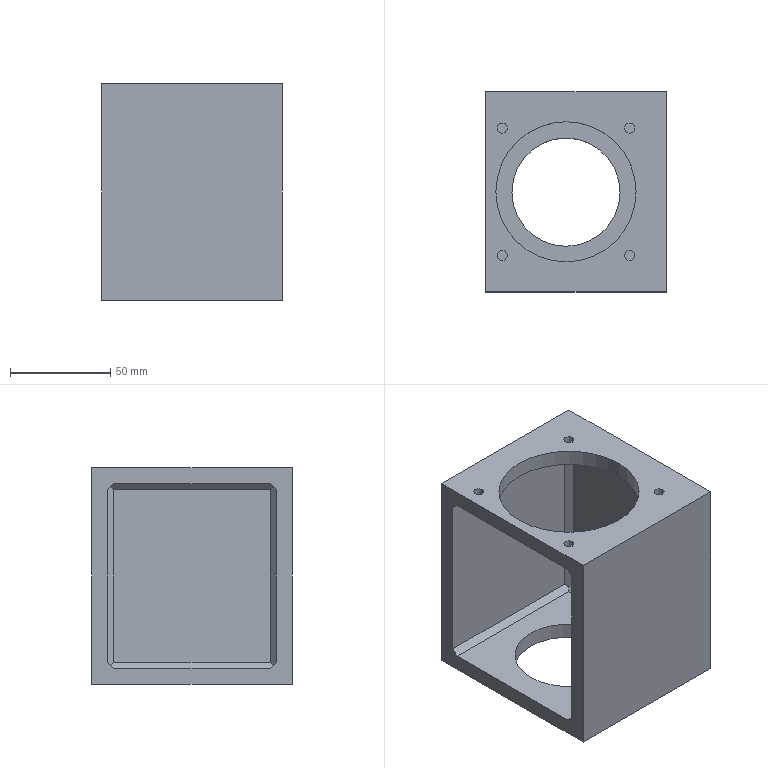Part | Creo | features CURVE 4, DATUM PLANE 3, CUT 2, PROTRUSION 2, CHAMFER 1, COORDINATE SYSTEM 1 | 1 solid | 31 faces | box 90 x 100 x 108 mm | volume 291545 mm3 | plane 19 | cylinder 12 | commonest cylinder face diameters 5 x8 54 x2 70 x2
STEP:
#1=CARTESIAN_POINT('',(0.,0.,0.));
#2=DIRECTION('',(0.,0.,1.));
#3=DIRECTION('',(1.,0.,0.));
#4=AXIS2_PLACEMENT_3D('',#1,#2,#3);
#5=CARTESIAN_POINT('',(-45.,50.,-54.));
#6=VERTEX_POINT('',#5);
#7=CARTESIAN_POINT('',(-45.,-50.,-54.));
#8=VERTEX_POINT('',#7);
#9=CARTESIAN_POINT('',(-45.,50.,-54.));
#10=DIRECTION('',(0.,-1.,0.));
#11=VECTOR('',#10,100.);
#12=LINE('',#9,#11);
#13=EDGE_CURVE('',#6,#8,#12,.T.);
#14=ORIENTED_EDGE('',*,*,#13,.T.);
#15=CARTESIAN_POINT('',(45.,-50.,-54.));
#16=VERTEX_POINT('',#15);
#17=CARTESIAN_POINT('',(-45.,-50.,-54.));
#18=DIRECTION('',(1.,0.,0.));
#19=VECTOR('',#18,90.);
#20=LINE('',#17,#19);
#21=EDGE_CURVE('',#8,#16,#20,.T.);
#22=ORIENTED_EDGE('',*,*,#21,.T.);
#23=CARTESIAN_POINT('',(45.,50.,-54.));
#24=VERTEX_POINT('',#23);
#25=CARTESIAN_POINT('',(45.,-50.,-54.));
#26=DIRECTION('',(0.,1.,0.));
#27=VECTOR('',#26,100.);
#28=LINE('',#25,#27);
#29=EDGE_CURVE('',#16,#24,#28,.T.);
#30=ORIENTED_EDGE('',*,*,#29,.T.);
#31=CARTESIAN_POINT('',(45.,50.,-54.));
#32=DIRECTION('',(-1.,0.,0.));
#33=VECTOR('',#32,90.);
#34=LINE('',#31,#33);
#35=EDGE_CURVE('',#24,#6,#34,.T.);
#36=ORIENTED_EDGE('',*,*,#35,.T.);
#37=EDGE_LOOP('',(#14,#22,#30,#36));
#38=FACE_OUTER_BOUND('',#37,.F.);
#39=CARTESIAN_POINT('',(-32.,0.,-54.));
#40=VERTEX_POINT('',#39);
#41=CARTESIAN_POINT('',(22.,0.,-54.));
#42=VERTEX_POINT('',#41);
#43=CARTESIAN_POINT('',(-5.,0.,-54.));
#44=DIRECTION('',(0.,0.,1.));
#45=DIRECTION('',(-1.,0.,0.));
#46=AXIS2_PLACEMENT_3D('',#43,#44,#45);
#47=CIRCLE('',#46,27.);
#48=EDGE_CURVE('',#40,#42,#47,.T.);
#49=ORIENTED_EDGE('',*,*,#48,.F.);
#50=CARTESIAN_POINT('',(-5.,0.,-54.));
#51=DIRECTION('',(0.,0.,1.));
#52=DIRECTION('',(1.,0.,0.));
#53=AXIS2_PLACEMENT_3D('',#50,#51,#52);
#54=CIRCLE('',#53,27.);
#55=EDGE_CURVE('',#42,#40,#54,.T.);
#56=ORIENTED_EDGE('',*,*,#55,.F.);
#57=EDGE_LOOP('',(#49,#56));
#58=FACE_BOUND('',#57,.F.);
#59=CARTESIAN_POINT('',(0.,0.,-54.));
#60=DIRECTION('',(0.,0.,1.));
#61=DIRECTION('',(1.,0.,0.));
#62=AXIS2_PLACEMENT_3D('',#59,#60,#61);
#63=PLANE('',#62);
#64=ADVANCED_FACE('',(#38,#58),#63,.F.);
#65=ORIENTED_EDGE('',*,*,#48,.T.);
#66=CARTESIAN_POINT('',(22.,0.,-46.));
#67=VERTEX_POINT('',#66);
#68=CARTESIAN_POINT('',(22.,0.,-54.));
#69=DIRECTION('',(0.,0.,1.));
#70=VECTOR('',#69,8.);
#71=LINE('',#68,#70);
#72=EDGE_CURVE('',#42,#67,#71,.T.);
#73=ORIENTED_EDGE('',*,*,#72,.T.);
#74=CARTESIAN_POINT('',(-32.,0.,-46.));
#75=VERTEX_POINT('',#74);
#76=CARTESIAN_POINT('',(-5.,0.,-46.));
#77=DIRECTION('',(0.,0.,1.));
#78=DIRECTION('',(-1.,0.,0.));
#79=AXIS2_PLACEMENT_3D('',#76,#77,#78);
#80=CIRCLE('',#79,27.);
#81=EDGE_CURVE('',#75,#67,#80,.T.);
#82=ORIENTED_EDGE('',*,*,#81,.F.);
#83=CARTESIAN_POINT('',(-32.,0.,-54.));
#84=DIRECTION('',(0.,0.,1.));
#85=VECTOR('',#84,8.);
#86=LINE('',#83,#85);
#87=EDGE_CURVE('',#40,#75,#86,.T.);
#88=ORIENTED_EDGE('',*,*,#87,.F.);
#89=EDGE_LOOP('',(#65,#73,#82,#88));
#90=FACE_OUTER_BOUND('',#89,.F.);
#91=CARTESIAN_POINT('',(-5.,0.,-54.));
#92=DIRECTION('',(0.,0.,-1.));
#93=DIRECTION('',(-1.,0.,0.));
#94=AXIS2_PLACEMENT_3D('',#91,#92,#93);
#95=CYLINDRICAL_SURFACE('',#94,27.);
#96=ADVANCED_FACE('',(#90),#95,.F.);
#97=ORIENTED_EDGE('',*,*,#55,.T.);
#98=ORIENTED_EDGE('',*,*,#87,.T.);
#99=CARTESIAN_POINT('',(-5.,0.,-46.));
#100=DIRECTION('',(0.,0.,1.));
#101=DIRECTION('',(1.,0.,0.));
#102=AXIS2_PLACEMENT_3D('',#99,#100,#101);
#103=CIRCLE('',#102,27.);
#104=EDGE_CURVE('',#67,#75,#103,.T.);
#105=ORIENTED_EDGE('',*,*,#104,.F.);
#106=ORIENTED_EDGE('',*,*,#72,.F.);
#107=EDGE_LOOP('',(#97,#98,#105,#106));
#108=FACE_OUTER_BOUND('',#107,.F.);
#109=CARTESIAN_POINT('',(-5.,0.,-54.));
#110=DIRECTION('',(0.,0.,-1.));
#111=DIRECTION('',(-1.,0.,0.));
#112=AXIS2_PLACEMENT_3D('',#109,#110,#111);
#113=CYLINDRICAL_SURFACE('',#112,27.);
#114=ADVANCED_FACE('',(#108),#113,.F.);
#115=CARTESIAN_POINT('',(-45.,-39.,-46.));
#116=VERTEX_POINT('',#115);
#117=CARTESIAN_POINT('',(34.,-39.,-46.));
#118=VERTEX_POINT('',#117);
#119=CARTESIAN_POINT('',(-45.,-39.,-46.));
#120=DIRECTION('',(1.,0.,0.));
#121=VECTOR('',#120,79.);
#122=LINE('',#119,#121);
#123=EDGE_CURVE('',#116,#118,#122,.T.);
#124=ORIENTED_EDGE('',*,*,#123,.F.);
#125=CARTESIAN_POINT('',(-45.,39.,-46.));
#126=VERTEX_POINT('',#125);
#127=CARTESIAN_POINT('',(-45.,39.,-46.));
#128=DIRECTION('',(0.,-1.,0.));
#129=VECTOR('',#128,78.);
#130=LINE('',#127,#129);
#131=EDGE_CURVE('',#126,#116,#130,.T.);
#132=ORIENTED_EDGE('',*,*,#131,.F.);
#133=CARTESIAN_POINT('',(34.,39.,-46.));
#134=VERTEX_POINT('',#133);
#135=CARTESIAN_POINT('',(-45.,39.,-46.));
#136=DIRECTION('',(1.,0.,0.));
#137=VECTOR('',#136,79.);
#138=LINE('',#135,#137);
#139=EDGE_CURVE('',#126,#134,#138,.T.);
#140=ORIENTED_EDGE('',*,*,#139,.T.);
#141=CARTESIAN_POINT('',(34.,-39.,-46.));
#142=DIRECTION('',(0.,1.,0.));
#143=VECTOR('',#142,78.);
#144=LINE('',#141,#143);
#145=EDGE_CURVE('',#118,#134,#144,.T.);
#146=ORIENTED_EDGE('',*,*,#145,.F.);
#147=EDGE_LOOP('',(#124,#132,#140,#146));
#148=FACE_OUTER_BOUND('',#147,.F.);
#149=ORIENTED_EDGE('',*,*,#81,.T.);
#150=ORIENTED_EDGE('',*,*,#104,.T.);
#151=EDGE_LOOP('',(#149,#150));
#152=FACE_BOUND('',#151,.F.);
#153=CARTESIAN_POINT('',(-45.,42.,-46.));
#154=DIRECTION('',(0.,0.,-1.));
#155=DIRECTION('',(0.,-1.,0.));
#156=AXIS2_PLACEMENT_3D('',#153,#154,#155);
#157=PLANE('',#156);
#158=ADVANCED_FACE('',(#148,#152),#157,.F.);
#159=ORIENTED_EDGE('',*,*,#123,.T.);
#160=CARTESIAN_POINT('',(35.5,-40.5,-44.5));
#161=VERTEX_POINT('',#160);
#162=CARTESIAN_POINT('',(35.5,-40.5,-44.5));
#163=DIRECTION('',(-0.5774,0.5774,-0.5774));
#164=VECTOR('',#163,2.598);
#165=LINE('',#162,#164);
#166=EDGE_CURVE('',#161,#118,#165,.T.);
#167=ORIENTED_EDGE('',*,*,#166,.F.);
#168=CARTESIAN_POINT('',(34.,-42.,-43.));
#169=VERTEX_POINT('',#168);
#170=CARTESIAN_POINT('',(34.,-42.,-43.));
#171=DIRECTION('',(0.5774,0.5774,-0.5774));
#172=VECTOR('',#171,2.598);
#173=LINE('',#170,#172);
#174=EDGE_CURVE('',#169,#161,#173,.T.);
#175=ORIENTED_EDGE('',*,*,#174,.F.);
#176=CARTESIAN_POINT('',(-45.,-42.,-43.));
#177=VERTEX_POINT('',#176);
#178=CARTESIAN_POINT('',(-45.,-42.,-43.));
#179=DIRECTION('',(1.,0.,0.));
#180=VECTOR('',#179,79.);
#181=LINE('',#178,#180);
#182=EDGE_CURVE('',#177,#169,#181,.T.);
#183=ORIENTED_EDGE('',*,*,#182,.F.);
#184=CARTESIAN_POINT('',(-45.,-42.,-43.));
#185=DIRECTION('',(0.,0.7071,-0.7071));
#186=VECTOR('',#185,4.243);
#187=LINE('',#184,#186);
#188=EDGE_CURVE('',#177,#116,#187,.T.);
#189=ORIENTED_EDGE('',*,*,#188,.T.);
#190=EDGE_LOOP('',(#159,#167,#175,#183,#189));
#191=FACE_OUTER_BOUND('',#190,.F.);
#192=CARTESIAN_POINT('',(-4.,-40.5,-44.5));
#193=DIRECTION('',(0.,0.7071,0.7071));
#194=DIRECTION('',(0.,-0.7071,0.7071));
#195=AXIS2_PLACEMENT_3D('',#192,#193,#194);
#196=PLANE('',#195);
#197=ADVANCED_FACE('',(#191),#196,.T.);
#198=ORIENTED_EDGE('',*,*,#145,.T.);
#199=CARTESIAN_POINT('',(35.5,40.5,-44.5));
#200=VERTEX_POINT('',#199);
#201=CARTESIAN_POINT('',(34.,39.,-46.));
#202=DIRECTION('',(0.5774,0.5774,0.5774));
#203=VECTOR('',#202,2.598);
#204=LINE('',#201,#203);
#205=EDGE_CURVE('',#134,#200,#204,.T.);
#206=ORIENTED_EDGE('',*,*,#205,.T.);
#207=CARTESIAN_POINT('',(37.,39.,-43.));
#208=VERTEX_POINT('',#207);
#209=CARTESIAN_POINT('',(37.,39.,-43.));
#210=DIRECTION('',(-0.5774,0.5774,-0.5774));
#211=VECTOR('',#210,2.598);
#212=LINE('',#209,#211);
#213=EDGE_CURVE('',#208,#200,#212,.T.);
#214=ORIENTED_EDGE('',*,*,#213,.F.);
#215=CARTESIAN_POINT('',(37.,-39.,-43.));
#216=VERTEX_POINT('',#215);
#217=CARTESIAN_POINT('',(37.,-39.,-43.));
#218=DIRECTION('',(0.,1.,0.));
#219=VECTOR('',#218,78.);
#220=LINE('',#217,#219);
#221=EDGE_CURVE('',#216,#208,#220,.T.);
#222=ORIENTED_EDGE('',*,*,#221,.F.);
#223=CARTESIAN_POINT('',(37.,-39.,-43.));
#224=DIRECTION('',(-0.5774,-0.5774,-0.5774));
#225=VECTOR('',#224,2.598);
#226=LINE('',#223,#225);
#227=EDGE_CURVE('',#216,#161,#226,.T.);
#228=ORIENTED_EDGE('',*,*,#227,.T.);
#229=ORIENTED_EDGE('',*,*,#166,.T.);
#230=EDGE_LOOP('',(#198,#206,#214,#222,#228,#229));
#231=FACE_OUTER_BOUND('',#230,.F.);
#232=CARTESIAN_POINT('',(35.5,0.,-44.5));
#233=DIRECTION('',(-0.7071,0.,0.7071));
#234=DIRECTION('',(0.7071,0.,0.7071));
#235=AXIS2_PLACEMENT_3D('',#232,#233,#234);
#236=PLANE('',#235);
#237=ADVANCED_FACE('',(#231),#236,.T.);
#238=CARTESIAN_POINT('',(-45.,42.,-43.));
#239=VERTEX_POINT('',#238);
#240=CARTESIAN_POINT('',(34.,42.,-43.));
#241=VERTEX_POINT('',#240);
#242=CARTESIAN_POINT('',(-45.,42.,-43.));
#243=DIRECTION('',(1.,0.,0.));
#244=VECTOR('',#243,79.);
#245=LINE('',#242,#244);
#246=EDGE_CURVE('',#239,#241,#245,.T.);
#247=ORIENTED_EDGE('',*,*,#246,.T.);
#248=CARTESIAN_POINT('',(35.5,40.5,-44.5));
#249=DIRECTION('',(-0.5774,0.5774,0.5774));
#250=VECTOR('',#249,2.598);
#251=LINE('',#248,#250);
#252=EDGE_CURVE('',#200,#241,#251,.T.);
#253=ORIENTED_EDGE('',*,*,#252,.F.);
#254=ORIENTED_EDGE('',*,*,#205,.F.);
#255=ORIENTED_EDGE('',*,*,#139,.F.);
#256=CARTESIAN_POINT('',(-45.,39.,-46.));
#257=DIRECTION('',(0.,0.7071,0.7071));
#258=VECTOR('',#257,4.243);
#259=LINE('',#256,#258);
#260=EDGE_CURVE('',#126,#239,#259,.T.);
#261=ORIENTED_EDGE('',*,*,#260,.T.);
#262=EDGE_LOOP('',(#247,#253,#254,#255,#261));
#263=FACE_OUTER_BOUND('',#262,.F.);
#264=CARTESIAN_POINT('',(-4.,40.5,-44.5));
#265=DIRECTION('',(0.,-0.7071,0.7071));
#266=DIRECTION('',(0.,-0.7071,-0.7071));
#267=AXIS2_PLACEMENT_3D('',#264,#265,#266);
#268=PLANE('',#267);
#269=ADVANCED_FACE('',(#263),#268,.T.);
#270=CARTESIAN_POINT('',(34.,42.,43.));
#271=VERTEX_POINT('',#270);
#272=CARTESIAN_POINT('',(34.,42.,-43.));
#273=DIRECTION('',(0.,0.,1.));
#274=VECTOR('',#273,86.);
#275=LINE('',#272,#274);
#276=EDGE_CURVE('',#241,#271,#275,.T.);
#277=ORIENTED_EDGE('',*,*,#276,.F.);
#278=ORIENTED_EDGE('',*,*,#246,.F.);
#279=CARTESIAN_POINT('',(-45.,42.,43.));
#280=VERTEX_POINT('',#279);
#281=CARTESIAN_POINT('',(-45.,42.,43.));
#282=DIRECTION('',(0.,0.,-1.));
#283=VECTOR('',#282,86.);
#284=LINE('',#281,#283);
#285=EDGE_CURVE('',#280,#239,#284,.T.);
#286=ORIENTED_EDGE('',*,*,#285,.F.);
#287=CARTESIAN_POINT('',(-45.,42.,43.));
#288=DIRECTION('',(1.,0.,0.));
#289=VECTOR('',#288,79.);
#290=LINE('',#287,#289);
#291=EDGE_CURVE('',#280,#271,#290,.T.);
#292=ORIENTED_EDGE('',*,*,#291,.T.);
#293=EDGE_LOOP('',(#277,#278,#286,#292));
#294=FACE_OUTER_BOUND('',#293,.F.);
#295=CARTESIAN_POINT('',(-45.,42.,46.));
#296=DIRECTION('',(0.,1.,0.));
#297=DIRECTION('',(0.,0.,-1.));
#298=AXIS2_PLACEMENT_3D('',#295,#296,#297);
#299=PLANE('',#298);
#300=ADVANCED_FACE('',(#294),#299,.F.);
#301=CARTESIAN_POINT('',(37.,39.,43.));
#302=VERTEX_POINT('',#301);
#303=CARTESIAN_POINT('',(37.,39.,-43.));
#304=DIRECTION('',(0.,0.,1.));
#305=VECTOR('',#304,86.);
#306=LINE('',#303,#305);
#307=EDGE_CURVE('',#208,#302,#306,.T.);
#308=ORIENTED_EDGE('',*,*,#307,.F.);
#309=ORIENTED_EDGE('',*,*,#213,.T.);
#310=ORIENTED_EDGE('',*,*,#252,.T.);
#311=ORIENTED_EDGE('',*,*,#276,.T.);
#312=CARTESIAN_POINT('',(35.5,40.5,44.5));
#313=VERTEX_POINT('',#312);
#314=CARTESIAN_POINT('',(34.,42.,43.));
#315=DIRECTION('',(0.5774,-0.5774,0.5774));
#316=VECTOR('',#315,2.598);
#317=LINE('',#314,#316);
#318=EDGE_CURVE('',#271,#313,#317,.T.);
#319=ORIENTED_EDGE('',*,*,#318,.T.);
#320=CARTESIAN_POINT('',(35.5,40.5,44.5));
#321=DIRECTION('',(0.5774,-0.5774,-0.5774));
#322=VECTOR('',#321,2.598);
#323=LINE('',#320,#322);
#324=EDGE_CURVE('',#313,#302,#323,.T.);
#325=ORIENTED_EDGE('',*,*,#324,.T.);
#326=EDGE_LOOP('',(#308,#309,#310,#311,#319,#325));
#327=FACE_OUTER_BOUND('',#326,.F.);
#328=CARTESIAN_POINT('',(35.5,40.5,0.));
#329=DIRECTION('',(-0.7071,-0.7071,0.));
#330=DIRECTION('',(0.7071,-0.7071,0.));
#331=AXIS2_PLACEMENT_3D('',#328,#329,#330);
#332=PLANE('',#331);
#333=ADVANCED_FACE('',(#327),#332,.T.);
#334=ORIENTED_EDGE('',*,*,#307,.T.);
#335=CARTESIAN_POINT('',(37.,-39.,43.));
#336=VERTEX_POINT('',#335);
#337=CARTESIAN_POINT('',(37.,39.,43.));
#338=DIRECTION('',(0.,-1.,0.));
#339=VECTOR('',#338,78.);
#340=LINE('',#337,#339);
#341=EDGE_CURVE('',#302,#336,#340,.T.);
#342=ORIENTED_EDGE('',*,*,#341,.T.);
#343=CARTESIAN_POINT('',(37.,-39.,43.));
#344=DIRECTION('',(0.,0.,-1.));
#345=VECTOR('',#344,86.);
#346=LINE('',#343,#345);
#347=EDGE_CURVE('',#336,#216,#346,.T.);
#348=ORIENTED_EDGE('',*,*,#347,.T.);
#349=ORIENTED_EDGE('',*,*,#221,.T.);
#350=EDGE_LOOP('',(#334,#342,#348,#349));
#351=FACE_OUTER_BOUND('',#350,.F.);
#352=CARTESIAN_POINT('',(37.,0.,-54.));
#353=DIRECTION('',(-1.,0.,0.));
#354=DIRECTION('',(0.,0.,1.));
#355=AXIS2_PLACEMENT_3D('',#352,#353,#354);
#356=PLANE('',#355);
#357=ADVANCED_FACE('',(#351),#356,.T.);
#358=ORIENTED_EDGE('',*,*,#341,.F.);
#359=ORIENTED_EDGE('',*,*,#324,.F.);
#360=CARTESIAN_POINT('',(34.,39.,46.));
#361=VERTEX_POINT('',#360);
#362=CARTESIAN_POINT('',(34.,39.,46.));
#363=DIRECTION('',(0.5774,0.5774,-0.5774));
#364=VECTOR('',#363,2.598);
#365=LINE('',#362,#364);
#366=EDGE_CURVE('',#361,#313,#365,.T.);
#367=ORIENTED_EDGE('',*,*,#366,.F.);
#368=CARTESIAN_POINT('',(34.,-39.,46.));
#369=VERTEX_POINT('',#368);
#370=CARTESIAN_POINT('',(34.,39.,46.));
#371=DIRECTION('',(0.,-1.,0.));
#372=VECTOR('',#371,78.);
#373=LINE('',#370,#372);
#374=EDGE_CURVE('',#361,#369,#373,.T.);
#375=ORIENTED_EDGE('',*,*,#374,.T.);
#376=CARTESIAN_POINT('',(35.5,-40.5,44.5));
#377=VERTEX_POINT('',#376);
#378=CARTESIAN_POINT('',(34.,-39.,46.));
#379=DIRECTION('',(0.5774,-0.5774,-0.5774));
#380=VECTOR('',#379,2.598);
#381=LINE('',#378,#380);
#382=EDGE_CURVE('',#369,#377,#381,.T.);
#383=ORIENTED_EDGE('',*,*,#382,.T.);
#384=CARTESIAN_POINT('',(37.,-39.,43.));
#385=DIRECTION('',(-0.5774,-0.5774,0.5774));
#386=VECTOR('',#385,2.598);
#387=LINE('',#384,#386);
#388=EDGE_CURVE('',#336,#377,#387,.T.);
#389=ORIENTED_EDGE('',*,*,#388,.F.);
#390=EDGE_LOOP('',(#358,#359,#367,#375,#383,#389));
#391=FACE_OUTER_BOUND('',#390,.F.);
#392=CARTESIAN_POINT('',(35.5,0.,44.5));
#393=DIRECTION('',(-0.7071,0.,-0.7071));
#394=DIRECTION('',(0.7071,0.,-0.7071));
#395=AXIS2_PLACEMENT_3D('',#392,#393,#394);
#396=PLANE('',#395);
#397=ADVANCED_FACE('',(#391),#396,.T.);
#398=CARTESIAN_POINT('',(-45.,39.,46.));
#399=VERTEX_POINT('',#398);
#400=CARTESIAN_POINT('',(-45.,39.,46.));
#401=DIRECTION('',(1.,0.,0.));
#402=VECTOR('',#401,79.);
#403=LINE('',#400,#402);
#404=EDGE_CURVE('',#399,#361,#403,.T.);
#405=ORIENTED_EDGE('',*,*,#404,.T.);
#406=ORIENTED_EDGE('',*,*,#366,.T.);
#407=ORIENTED_EDGE('',*,*,#318,.F.);
#408=ORIENTED_EDGE('',*,*,#291,.F.);
#409=CARTESIAN_POINT('',(-45.,42.,43.));
#410=DIRECTION('',(0.,-0.7071,0.7071));
#411=VECTOR('',#410,4.243);
#412=LINE('',#409,#411);
#413=EDGE_CURVE('',#280,#399,#412,.T.);
#414=ORIENTED_EDGE('',*,*,#413,.T.);
#415=EDGE_LOOP('',(#405,#406,#407,#408,#414));
#416=FACE_OUTER_BOUND('',#415,.F.);
#417=CARTESIAN_POINT('',(-4.,40.5,44.5));
#418=DIRECTION('',(0.,-0.7071,-0.7071));
#419=DIRECTION('',(0.,0.7071,-0.7071));
#420=AXIS2_PLACEMENT_3D('',#417,#418,#419);
#421=PLANE('',#420);
#422=ADVANCED_FACE('',(#416),#421,.T.);
#423=ORIENTED_EDGE('',*,*,#404,.F.);
#424=CARTESIAN_POINT('',(-45.,-39.,46.));
#425=VERTEX_POINT('',#424);
#426=CARTESIAN_POINT('',(-45.,-39.,46.));
#427=DIRECTION('',(0.,1.,0.));
#428=VECTOR('',#427,78.);
#429=LINE('',#426,#428);
#430=EDGE_CURVE('',#425,#399,#429,.T.);
#431=ORIENTED_EDGE('',*,*,#430,.F.);
#432=CARTESIAN_POINT('',(-45.,-39.,46.));
#433=DIRECTION('',(1.,0.,0.));
#434=VECTOR('',#433,79.);
#435=LINE('',#432,#434);
#436=EDGE_CURVE('',#425,#369,#435,.T.);
#437=ORIENTED_EDGE('',*,*,#436,.T.);
#438=ORIENTED_EDGE('',*,*,#374,.F.);
#439=EDGE_LOOP('',(#423,#431,#437,#438));
#440=FACE_OUTER_BOUND('',#439,.F.);
#441=CARTESIAN_POINT('',(29.32,31.82,46.));
#442=VERTEX_POINT('',#441);
#443=CARTESIAN_POINT('',(24.32,31.82,46.));
#444=VERTEX_POINT('',#443);
#445=CARTESIAN_POINT('',(26.82,31.82,46.));
#446=DIRECTION('',(0.,0.,1.));
#447=DIRECTION('',(1.,0.,0.));
#448=AXIS2_PLACEMENT_3D('',#445,#446,#447);
#449=CIRCLE('',#448,2.5);
#450=EDGE_CURVE('',#442,#444,#449,.T.);
#451=ORIENTED_EDGE('',*,*,#450,.F.);
#452=CARTESIAN_POINT('',(26.82,31.82,46.));
#453=DIRECTION('',(0.,0.,1.));
#454=DIRECTION('',(-1.,0.,0.));
#455=AXIS2_PLACEMENT_3D('',#452,#453,#454);
#456=CIRCLE('',#455,2.5);
#457=EDGE_CURVE('',#444,#442,#456,.T.);
#458=ORIENTED_EDGE('',*,*,#457,.F.);
#459=EDGE_LOOP('',(#451,#458));
#460=FACE_BOUND('',#459,.F.);
#461=CARTESIAN_POINT('',(-34.32,31.82,46.));
#462=VERTEX_POINT('',#461);
#463=CARTESIAN_POINT('',(-39.32,31.82,46.));
#464=VERTEX_POINT('',#463);
#465=CARTESIAN_POINT('',(-36.82,31.82,46.));
#466=DIRECTION('',(0.,0.,1.));
#467=DIRECTION('',(1.,0.,0.));
#468=AXIS2_PLACEMENT_3D('',#465,#466,#467);
#469=CIRCLE('',#468,2.5);
#470=EDGE_CURVE('',#462,#464,#469,.T.);
#471=ORIENTED_EDGE('',*,*,#470,.F.);
#472=CARTESIAN_POINT('',(-36.82,31.82,46.));
#473=DIRECTION('',(0.,0.,1.));
#474=DIRECTION('',(-1.,0.,0.));
#475=AXIS2_PLACEMENT_3D('',#472,#473,#474);
#476=CIRCLE('',#475,2.5);
#477=EDGE_CURVE('',#464,#462,#476,.T.);
#478=ORIENTED_EDGE('',*,*,#477,.F.);
#479=EDGE_LOOP('',(#471,#478));
#480=FACE_BOUND('',#479,.F.);
#481=CARTESIAN_POINT('',(-34.32,-31.82,46.));
#482=VERTEX_POINT('',#481);
#483=CARTESIAN_POINT('',(-39.32,-31.82,46.));
#484=VERTEX_POINT('',#483);
#485=CARTESIAN_POINT('',(-36.82,-31.82,46.));
#486=DIRECTION('',(0.,0.,1.));
#487=DIRECTION('',(1.,0.,0.));
#488=AXIS2_PLACEMENT_3D('',#485,#486,#487);
#489=CIRCLE('',#488,2.5);
#490=EDGE_CURVE('',#482,#484,#489,.T.);
#491=ORIENTED_EDGE('',*,*,#490,.F.);
#492=CARTESIAN_POINT('',(-36.82,-31.82,46.));
#493=DIRECTION('',(0.,0.,1.));
#494=DIRECTION('',(-1.,0.,0.));
#495=AXIS2_PLACEMENT_3D('',#492,#493,#494);
#496=CIRCLE('',#495,2.5);
#497=EDGE_CURVE('',#484,#482,#496,.T.);
#498=ORIENTED_EDGE('',*,*,#497,.F.);
#499=EDGE_LOOP('',(#491,#498));
#500=FACE_BOUND('',#499,.F.);
#501=CARTESIAN_POINT('',(29.32,-31.82,46.));
#502=VERTEX_POINT('',#501);
#503=CARTESIAN_POINT('',(24.32,-31.82,46.));
#504=VERTEX_POINT('',#503);
#505=CARTESIAN_POINT('',(26.82,-31.82,46.));
#506=DIRECTION('',(0.,0.,1.));
#507=DIRECTION('',(1.,0.,0.));
#508=AXIS2_PLACEMENT_3D('',#505,#506,#507);
#509=CIRCLE('',#508,2.5);
#510=EDGE_CURVE('',#502,#504,#509,.T.);
#511=ORIENTED_EDGE('',*,*,#510,.F.);
#512=CARTESIAN_POINT('',(26.82,-31.82,46.));
#513=DIRECTION('',(0.,0.,1.));
#514=DIRECTION('',(-1.,0.,0.));
#515=AXIS2_PLACEMENT_3D('',#512,#513,#514);
#516=CIRCLE('',#515,2.5);
#517=EDGE_CURVE('',#504,#502,#516,.T.);
#518=ORIENTED_EDGE('',*,*,#517,.F.);
#519=EDGE_LOOP('',(#511,#518));
#520=FACE_BOUND('',#519,.F.);
#521=CARTESIAN_POINT('',(-40.,0.,46.));
#522=VERTEX_POINT('',#521);
#523=CARTESIAN_POINT('',(30.,0.,46.));
#524=VERTEX_POINT('',#523);
#525=CARTESIAN_POINT('',(-5.,0.,46.));
#526=DIRECTION('',(0.,0.,1.));
#527=DIRECTION('',(-1.,0.,0.));
#528=AXIS2_PLACEMENT_3D('',#525,#526,#527);
#529=CIRCLE('',#528,35.);
#530=EDGE_CURVE('',#522,#524,#529,.T.);
#531=ORIENTED_EDGE('',*,*,#530,.F.);
#532=CARTESIAN_POINT('',(-5.,0.,46.));
#533=DIRECTION('',(0.,0.,1.));
#534=DIRECTION('',(1.,0.,0.));
#535=AXIS2_PLACEMENT_3D('',#532,#533,#534);
#536=CIRCLE('',#535,35.);
#537=EDGE_CURVE('',#524,#522,#536,.T.);
#538=ORIENTED_EDGE('',*,*,#537,.F.);
#539=EDGE_LOOP('',(#531,#538));
#540=FACE_BOUND('',#539,.F.);
#541=CARTESIAN_POINT('',(-45.,-42.,46.));
#542=DIRECTION('',(0.,0.,1.));
#543=DIRECTION('',(0.,1.,0.));
#544=AXIS2_PLACEMENT_3D('',#541,#542,#543);
#545=PLANE('',#544);
#546=ADVANCED_FACE('',(#440,#460,#480,#500,#520,#540),#545,.F.);
#547=ORIENTED_EDGE('',*,*,#530,.T.);
#548=CARTESIAN_POINT('',(30.,0.,54.));
#549=VERTEX_POINT('',#548);
#550=CARTESIAN_POINT('',(30.,0.,46.));
#551=DIRECTION('',(0.,0.,1.));
#552=VECTOR('',#551,8.);
#553=LINE('',#550,#552);
#554=EDGE_CURVE('',#524,#549,#553,.T.);
#555=ORIENTED_EDGE('',*,*,#554,.T.);
#556=CARTESIAN_POINT('',(-40.,0.,54.));
#557=VERTEX_POINT('',#556);
#558=CARTESIAN_POINT('',(-5.,0.,54.));
#559=DIRECTION('',(0.,0.,-1.));
#560=DIRECTION('',(1.,0.,0.));
#561=AXIS2_PLACEMENT_3D('',#558,#559,#560);
#562=CIRCLE('',#561,35.);
#563=EDGE_CURVE('',#549,#557,#562,.T.);
#564=ORIENTED_EDGE('',*,*,#563,.T.);
#565=CARTESIAN_POINT('',(-40.,0.,46.));
#566=DIRECTION('',(0.,0.,1.));
#567=VECTOR('',#566,8.);
#568=LINE('',#565,#567);
#569=EDGE_CURVE('',#522,#557,#568,.T.);
#570=ORIENTED_EDGE('',*,*,#569,.F.);
#571=EDGE_LOOP('',(#547,#555,#564,#570));
#572=FACE_OUTER_BOUND('',#571,.F.);
#573=CARTESIAN_POINT('',(-5.,0.,-54.));
#574=DIRECTION('',(0.,0.,1.));
#575=DIRECTION('',(1.,0.,0.));
#576=AXIS2_PLACEMENT_3D('',#573,#574,#575);
#577=CYLINDRICAL_SURFACE('',#576,35.);
#578=ADVANCED_FACE('',(#572),#577,.F.);
#579=ORIENTED_EDGE('',*,*,#537,.T.);
#580=ORIENTED_EDGE('',*,*,#569,.T.);
#581=CARTESIAN_POINT('',(-5.,0.,54.));
#582=DIRECTION('',(0.,0.,-1.));
#583=DIRECTION('',(-1.,0.,0.));
#584=AXIS2_PLACEMENT_3D('',#581,#582,#583);
#585=CIRCLE('',#584,35.);
#586=EDGE_CURVE('',#557,#549,#585,.T.);
#587=ORIENTED_EDGE('',*,*,#586,.T.);
#588=ORIENTED_EDGE('',*,*,#554,.F.);
#589=EDGE_LOOP('',(#579,#580,#587,#588));
#590=FACE_OUTER_BOUND('',#589,.F.);
#591=CARTESIAN_POINT('',(-5.,0.,-54.));
#592=DIRECTION('',(0.,0.,1.));
#593=DIRECTION('',(1.,0.,0.));
#594=AXIS2_PLACEMENT_3D('',#591,#592,#593);
#595=CYLINDRICAL_SURFACE('',#594,35.);
#596=ADVANCED_FACE('',(#590),#595,.F.);
#597=CARTESIAN_POINT('',(-45.,50.,54.));
#598=VERTEX_POINT('',#597);
#599=CARTESIAN_POINT('',(-45.,-50.,54.));
#600=VERTEX_POINT('',#599);
#601=CARTESIAN_POINT('',(-45.,50.,54.));
#602=DIRECTION('',(0.,-1.,0.));
#603=VECTOR('',#602,100.);
#604=LINE('',#601,#603);
#605=EDGE_CURVE('',#598,#600,#604,.T.);
#606=ORIENTED_EDGE('',*,*,#605,.F.);
#607=CARTESIAN_POINT('',(45.,50.,54.));
#608=VERTEX_POINT('',#607);
#609=CARTESIAN_POINT('',(45.,50.,54.));
#610=DIRECTION('',(-1.,0.,0.));
#611=VECTOR('',#610,90.);
#612=LINE('',#609,#611);
#613=EDGE_CURVE('',#608,#598,#612,.T.);
#614=ORIENTED_EDGE('',*,*,#613,.F.);
#615=CARTESIAN_POINT('',(45.,-50.,54.));
#616=VERTEX_POINT('',#615);
#617=CARTESIAN_POINT('',(45.,-50.,54.));
#618=DIRECTION('',(0.,1.,0.));
#619=VECTOR('',#618,100.);
#620=LINE('',#617,#619);
#621=EDGE_CURVE('',#616,#608,#620,.T.);
#622=ORIENTED_EDGE('',*,*,#621,.F.);
#623=CARTESIAN_POINT('',(-45.,-50.,54.));
#624=DIRECTION('',(1.,0.,0.));
#625=VECTOR('',#624,90.);
#626=LINE('',#623,#625);
#627=EDGE_CURVE('',#600,#616,#626,.T.);
#628=ORIENTED_EDGE('',*,*,#627,.F.);
#629=EDGE_LOOP('',(#606,#614,#622,#628));
#630=FACE_OUTER_BOUND('',#629,.F.);
#631=ORIENTED_EDGE('',*,*,#563,.F.);
#632=ORIENTED_EDGE('',*,*,#586,.F.);
#633=EDGE_LOOP('',(#631,#632));
#634=FACE_BOUND('',#633,.F.);
#635=CARTESIAN_POINT('',(29.32,31.82,54.));
#636=VERTEX_POINT('',#635);
#637=CARTESIAN_POINT('',(24.32,31.82,54.));
#638=VERTEX_POINT('',#637);
#639=CARTESIAN_POINT('',(26.82,31.82,54.));
#640=DIRECTION('',(0.,0.,1.));
#641=DIRECTION('',(1.,0.,0.));
#642=AXIS2_PLACEMENT_3D('',#639,#640,#641);
#643=CIRCLE('',#642,2.5);
#644=EDGE_CURVE('',#636,#638,#643,.T.);
#645=ORIENTED_EDGE('',*,*,#644,.T.);
#646=CARTESIAN_POINT('',(26.82,31.82,54.));
#647=DIRECTION('',(0.,0.,1.));
#648=DIRECTION('',(-1.,0.,0.));
#649=AXIS2_PLACEMENT_3D('',#646,#647,#648);
#650=CIRCLE('',#649,2.5);
#651=EDGE_CURVE('',#638,#636,#650,.T.);
#652=ORIENTED_EDGE('',*,*,#651,.T.);
#653=EDGE_LOOP('',(#645,#652));
#654=FACE_BOUND('',#653,.F.);
#655=CARTESIAN_POINT('',(-34.32,31.82,54.));
#656=VERTEX_POINT('',#655);
#657=CARTESIAN_POINT('',(-39.32,31.82,54.));
#658=VERTEX_POINT('',#657);
#659=CARTESIAN_POINT('',(-36.82,31.82,54.));
#660=DIRECTION('',(0.,0.,1.));
#661=DIRECTION('',(1.,0.,0.));
#662=AXIS2_PLACEMENT_3D('',#659,#660,#661);
#663=CIRCLE('',#662,2.5);
#664=EDGE_CURVE('',#656,#658,#663,.T.);
#665=ORIENTED_EDGE('',*,*,#664,.T.);
#666=CARTESIAN_POINT('',(-36.82,31.82,54.));
#667=DIRECTION('',(0.,0.,1.));
#668=DIRECTION('',(-1.,0.,0.));
#669=AXIS2_PLACEMENT_3D('',#666,#667,#668);
#670=CIRCLE('',#669,2.5);
#671=EDGE_CURVE('',#658,#656,#670,.T.);
#672=ORIENTED_EDGE('',*,*,#671,.T.);
#673=EDGE_LOOP('',(#665,#672));
#674=FACE_BOUND('',#673,.F.);
#675=CARTESIAN_POINT('',(-34.32,-31.82,54.));
#676=VERTEX_POINT('',#675);
#677=CARTESIAN_POINT('',(-39.32,-31.82,54.));
#678=VERTEX_POINT('',#677);
#679=CARTESIAN_POINT('',(-36.82,-31.82,54.));
#680=DIRECTION('',(0.,0.,1.));
#681=DIRECTION('',(1.,0.,0.));
#682=AXIS2_PLACEMENT_3D('',#679,#680,#681);
#683=CIRCLE('',#682,2.5);
#684=EDGE_CURVE('',#676,#678,#683,.T.);
#685=ORIENTED_EDGE('',*,*,#684,.T.);
#686=CARTESIAN_POINT('',(-36.82,-31.82,54.));
#687=DIRECTION('',(0.,0.,1.));
#688=DIRECTION('',(-1.,0.,0.));
#689=AXIS2_PLACEMENT_3D('',#686,#687,#688);
#690=CIRCLE('',#689,2.5);
#691=EDGE_CURVE('',#678,#676,#690,.T.);
#692=ORIENTED_EDGE('',*,*,#691,.T.);
#693=EDGE_LOOP('',(#685,#692));
#694=FACE_BOUND('',#693,.F.);
#695=CARTESIAN_POINT('',(29.32,-31.82,54.));
#696=VERTEX_POINT('',#695);
#697=CARTESIAN_POINT('',(24.32,-31.82,54.));
#698=VERTEX_POINT('',#697);
#699=CARTESIAN_POINT('',(26.82,-31.82,54.));
#700=DIRECTION('',(0.,0.,1.));
#701=DIRECTION('',(1.,0.,0.));
#702=AXIS2_PLACEMENT_3D('',#699,#700,#701);
#703=CIRCLE('',#702,2.5);
#704=EDGE_CURVE('',#696,#698,#703,.T.);
#705=ORIENTED_EDGE('',*,*,#704,.T.);
#706=CARTESIAN_POINT('',(26.82,-31.82,54.));
#707=DIRECTION('',(0.,0.,1.));
#708=DIRECTION('',(-1.,0.,0.));
#709=AXIS2_PLACEMENT_3D('',#706,#707,#708);
#710=CIRCLE('',#709,2.5);
#711=EDGE_CURVE('',#698,#696,#710,.T.);
#712=ORIENTED_EDGE('',*,*,#711,.T.);
#713=EDGE_LOOP('',(#705,#712));
#714=FACE_BOUND('',#713,.F.);
#715=CARTESIAN_POINT('',(0.,0.,54.));
#716=DIRECTION('',(0.,0.,1.));
#717=DIRECTION('',(1.,0.,0.));
#718=AXIS2_PLACEMENT_3D('',#715,#716,#717);
#719=PLANE('',#718);
#720=ADVANCED_FACE('',(#630,#634,#654,#674,#694,#714),#719,.T.);
#721=ORIENTED_EDGE('',*,*,#13,.F.);
#722=CARTESIAN_POINT('',(-45.,50.,-54.));
#723=DIRECTION('',(0.,0.,1.));
#724=VECTOR('',#723,108.);
#725=LINE('',#722,#724);
#726=EDGE_CURVE('',#6,#598,#725,.T.);
#727=ORIENTED_EDGE('',*,*,#726,.T.);
#728=ORIENTED_EDGE('',*,*,#605,.T.);
#729=CARTESIAN_POINT('',(-45.,-50.,-54.));
#730=DIRECTION('',(0.,0.,1.));
#731=VECTOR('',#730,108.);
#732=LINE('',#729,#731);
#733=EDGE_CURVE('',#8,#600,#732,.T.);
#734=ORIENTED_EDGE('',*,*,#733,.F.);
#735=EDGE_LOOP('',(#721,#727,#728,#734));
#736=FACE_OUTER_BOUND('',#735,.F.);
#737=ORIENTED_EDGE('',*,*,#285,.T.);
#738=ORIENTED_EDGE('',*,*,#260,.F.);
#739=ORIENTED_EDGE('',*,*,#131,.T.);
#740=ORIENTED_EDGE('',*,*,#188,.F.);
#741=CARTESIAN_POINT('',(-45.,-42.,43.));
#742=VERTEX_POINT('',#741);
#743=CARTESIAN_POINT('',(-45.,-42.,-43.));
#744=DIRECTION('',(0.,0.,1.));
#745=VECTOR('',#744,86.);
#746=LINE('',#743,#745);
#747=EDGE_CURVE('',#177,#742,#746,.T.);
#748=ORIENTED_EDGE('',*,*,#747,.T.);
#749=CARTESIAN_POINT('',(-45.,-39.,46.));
#750=DIRECTION('',(0.,-0.7071,-0.7071));
#751=VECTOR('',#750,4.243);
#752=LINE('',#749,#751);
#753=EDGE_CURVE('',#425,#742,#752,.T.);
#754=ORIENTED_EDGE('',*,*,#753,.F.);
#755=ORIENTED_EDGE('',*,*,#430,.T.);
#756=ORIENTED_EDGE('',*,*,#413,.F.);
#757=EDGE_LOOP('',(#737,#738,#739,#740,#748,#754,#755,#756));
#758=FACE_BOUND('',#757,.F.);
#759=CARTESIAN_POINT('',(-45.,50.,-54.));
#760=DIRECTION('',(-1.,0.,0.));
#761=DIRECTION('',(0.,-1.,0.));
#762=AXIS2_PLACEMENT_3D('',#759,#760,#761);
#763=PLANE('',#762);
#764=ADVANCED_FACE('',(#736,#758),#763,.T.);
#765=ORIENTED_EDGE('',*,*,#35,.F.);
#766=CARTESIAN_POINT('',(45.,50.,-54.));
#767=DIRECTION('',(0.,0.,1.));
#768=VECTOR('',#767,108.);
#769=LINE('',#766,#768);
#770=EDGE_CURVE('',#24,#608,#769,.T.);
#771=ORIENTED_EDGE('',*,*,#770,.T.);
#772=ORIENTED_EDGE('',*,*,#613,.T.);
#773=ORIENTED_EDGE('',*,*,#726,.F.);
#774=EDGE_LOOP('',(#765,#771,#772,#773));
#775=FACE_OUTER_BOUND('',#774,.F.);
#776=CARTESIAN_POINT('',(45.,50.,-54.));
#777=DIRECTION('',(0.,1.,0.));
#778=DIRECTION('',(-1.,0.,0.));
#779=AXIS2_PLACEMENT_3D('',#776,#777,#778);
#780=PLANE('',#779);
#781=ADVANCED_FACE('',(#775),#780,.T.);
#782=ORIENTED_EDGE('',*,*,#29,.F.);
#783=CARTESIAN_POINT('',(45.,-50.,-54.));
#784=DIRECTION('',(0.,0.,1.));
#785=VECTOR('',#784,108.);
#786=LINE('',#783,#785);
#787=EDGE_CURVE('',#16,#616,#786,.T.);
#788=ORIENTED_EDGE('',*,*,#787,.T.);
#789=ORIENTED_EDGE('',*,*,#621,.T.);
#790=ORIENTED_EDGE('',*,*,#770,.F.);
#791=EDGE_LOOP('',(#782,#788,#789,#790));
#792=FACE_OUTER_BOUND('',#791,.F.);
#793=CARTESIAN_POINT('',(45.,-50.,-54.));
#794=DIRECTION('',(1.,0.,0.));
#795=DIRECTION('',(0.,1.,0.));
#796=AXIS2_PLACEMENT_3D('',#793,#794,#795);
#797=PLANE('',#796);
#798=ADVANCED_FACE('',(#792),#797,.T.);
#799=ORIENTED_EDGE('',*,*,#21,.F.);
#800=ORIENTED_EDGE('',*,*,#733,.T.);
#801=ORIENTED_EDGE('',*,*,#627,.T.);
#802=ORIENTED_EDGE('',*,*,#787,.F.);
#803=EDGE_LOOP('',(#799,#800,#801,#802));
#804=FACE_OUTER_BOUND('',#803,.F.);
#805=CARTESIAN_POINT('',(-45.,-50.,-54.));
#806=DIRECTION('',(0.,-1.,0.));
#807=DIRECTION('',(1.,0.,0.));
#808=AXIS2_PLACEMENT_3D('',#805,#806,#807);
#809=PLANE('',#808);
#810=ADVANCED_FACE('',(#804),#809,.T.);
#811=CARTESIAN_POINT('',(34.,-42.,43.));
#812=VERTEX_POINT('',#811);
#813=CARTESIAN_POINT('',(-45.,-42.,43.));
#814=DIRECTION('',(1.,0.,0.));
#815=VECTOR('',#814,79.);
#816=LINE('',#813,#815);
#817=EDGE_CURVE('',#742,#812,#816,.T.);
#818=ORIENTED_EDGE('',*,*,#817,.F.);
#819=ORIENTED_EDGE('',*,*,#747,.F.);
#820=ORIENTED_EDGE('',*,*,#182,.T.);
#821=CARTESIAN_POINT('',(34.,-42.,43.));
#822=DIRECTION('',(0.,0.,-1.));
#823=VECTOR('',#822,86.);
#824=LINE('',#821,#823);
#825=EDGE_CURVE('',#812,#169,#824,.T.);
#826=ORIENTED_EDGE('',*,*,#825,.F.);
#827=EDGE_LOOP('',(#818,#819,#820,#826));
#828=FACE_OUTER_BOUND('',#827,.F.);
#829=CARTESIAN_POINT('',(-45.,-42.,-46.));
#830=DIRECTION('',(0.,-1.,0.));
#831=DIRECTION('',(0.,0.,1.));
#832=AXIS2_PLACEMENT_3D('',#829,#830,#831);
#833=PLANE('',#832);
#834=ADVANCED_FACE('',(#828),#833,.F.);
#835=ORIENTED_EDGE('',*,*,#817,.T.);
#836=CARTESIAN_POINT('',(35.5,-40.5,44.5));
#837=DIRECTION('',(-0.5774,-0.5774,-0.5774));
#838=VECTOR('',#837,2.598);
#839=LINE('',#836,#838);
#840=EDGE_CURVE('',#377,#812,#839,.T.);
#841=ORIENTED_EDGE('',*,*,#840,.F.);
#842=ORIENTED_EDGE('',*,*,#382,.F.);
#843=ORIENTED_EDGE('',*,*,#436,.F.);
#844=ORIENTED_EDGE('',*,*,#753,.T.);
#845=EDGE_LOOP('',(#835,#841,#842,#843,#844));
#846=FACE_OUTER_BOUND('',#845,.F.);
#847=CARTESIAN_POINT('',(-4.,-40.5,44.5));
#848=DIRECTION('',(0.,0.7071,-0.7071));
#849=DIRECTION('',(0.,0.7071,0.7071));
#850=AXIS2_PLACEMENT_3D('',#847,#848,#849);
#851=PLANE('',#850);
#852=ADVANCED_FACE('',(#846),#851,.T.);
#853=ORIENTED_EDGE('',*,*,#825,.T.);
#854=ORIENTED_EDGE('',*,*,#174,.T.);
#855=ORIENTED_EDGE('',*,*,#227,.F.);
#856=ORIENTED_EDGE('',*,*,#347,.F.);
#857=ORIENTED_EDGE('',*,*,#388,.T.);
#858=ORIENTED_EDGE('',*,*,#840,.T.);
#859=EDGE_LOOP('',(#853,#854,#855,#856,#857,#858));
#860=FACE_OUTER_BOUND('',#859,.F.);
#861=CARTESIAN_POINT('',(35.5,-40.5,0.));
#862=DIRECTION('',(-0.7071,0.7071,0.));
#863=DIRECTION('',(0.7071,0.7071,0.));
#864=AXIS2_PLACEMENT_3D('',#861,#862,#863);
#865=PLANE('',#864);
#866=ADVANCED_FACE('',(#860),#865,.T.);
#867=ORIENTED_EDGE('',*,*,#644,.F.);
#868=CARTESIAN_POINT('',(29.32,31.82,54.));
#869=DIRECTION('',(0.,0.,-1.));
#870=VECTOR('',#869,8.);
#871=LINE('',#868,#870);
#872=EDGE_CURVE('',#636,#442,#871,.T.);
#873=ORIENTED_EDGE('',*,*,#872,.T.);
#874=ORIENTED_EDGE('',*,*,#450,.T.);
#875=CARTESIAN_POINT('',(24.32,31.82,54.));
#876=DIRECTION('',(0.,0.,-1.));
#877=VECTOR('',#876,8.);
#878=LINE('',#875,#877);
#879=EDGE_CURVE('',#638,#444,#878,.T.);
#880=ORIENTED_EDGE('',*,*,#879,.F.);
#881=EDGE_LOOP('',(#867,#873,#874,#880));
#882=FACE_OUTER_BOUND('',#881,.F.);
#883=CARTESIAN_POINT('',(26.82,31.82,54.));
#884=DIRECTION('',(0.,0.,1.));
#885=DIRECTION('',(1.,0.,0.));
#886=AXIS2_PLACEMENT_3D('',#883,#884,#885);
#887=CYLINDRICAL_SURFACE('',#886,2.5);
#888=ADVANCED_FACE('',(#882),#887,.F.);
#889=ORIENTED_EDGE('',*,*,#651,.F.);
#890=ORIENTED_EDGE('',*,*,#879,.T.);
#891=ORIENTED_EDGE('',*,*,#457,.T.);
#892=ORIENTED_EDGE('',*,*,#872,.F.);
#893=EDGE_LOOP('',(#889,#890,#891,#892));
#894=FACE_OUTER_BOUND('',#893,.F.);
#895=CARTESIAN_POINT('',(26.82,31.82,54.));
#896=DIRECTION('',(0.,0.,1.));
#897=DIRECTION('',(1.,0.,0.));
#898=AXIS2_PLACEMENT_3D('',#895,#896,#897);
#899=CYLINDRICAL_SURFACE('',#898,2.5);
#900=ADVANCED_FACE('',(#894),#899,.F.);
#901=ORIENTED_EDGE('',*,*,#664,.F.);
#902=CARTESIAN_POINT('',(-34.32,31.82,54.));
#903=DIRECTION('',(0.,0.,-1.));
#904=VECTOR('',#903,8.);
#905=LINE('',#902,#904);
#906=EDGE_CURVE('',#656,#462,#905,.T.);
#907=ORIENTED_EDGE('',*,*,#906,.T.);
#908=ORIENTED_EDGE('',*,*,#470,.T.);
#909=CARTESIAN_POINT('',(-39.32,31.82,54.));
#910=DIRECTION('',(0.,0.,-1.));
#911=VECTOR('',#910,8.);
#912=LINE('',#909,#911);
#913=EDGE_CURVE('',#658,#464,#912,.T.);
#914=ORIENTED_EDGE('',*,*,#913,.F.);
#915=EDGE_LOOP('',(#901,#907,#908,#914));
#916=FACE_OUTER_BOUND('',#915,.F.);
#917=CARTESIAN_POINT('',(-36.82,31.82,54.));
#918=DIRECTION('',(0.,0.,1.));
#919=DIRECTION('',(1.,0.,0.));
#920=AXIS2_PLACEMENT_3D('',#917,#918,#919);
#921=CYLINDRICAL_SURFACE('',#920,2.5);
#922=ADVANCED_FACE('',(#916),#921,.F.);
#923=ORIENTED_EDGE('',*,*,#671,.F.);
#924=ORIENTED_EDGE('',*,*,#913,.T.);
#925=ORIENTED_EDGE('',*,*,#477,.T.);
#926=ORIENTED_EDGE('',*,*,#906,.F.);
#927=EDGE_LOOP('',(#923,#924,#925,#926));
#928=FACE_OUTER_BOUND('',#927,.F.);
#929=CARTESIAN_POINT('',(-36.82,31.82,54.));
#930=DIRECTION('',(0.,0.,1.));
#931=DIRECTION('',(1.,0.,0.));
#932=AXIS2_PLACEMENT_3D('',#929,#930,#931);
#933=CYLINDRICAL_SURFACE('',#932,2.5);
#934=ADVANCED_FACE('',(#928),#933,.F.);
#935=ORIENTED_EDGE('',*,*,#684,.F.);
#936=CARTESIAN_POINT('',(-34.32,-31.82,54.));
#937=DIRECTION('',(0.,0.,-1.));
#938=VECTOR('',#937,8.);
#939=LINE('',#936,#938);
#940=EDGE_CURVE('',#676,#482,#939,.T.);
#941=ORIENTED_EDGE('',*,*,#940,.T.);
#942=ORIENTED_EDGE('',*,*,#490,.T.);
#943=CARTESIAN_POINT('',(-39.32,-31.82,54.));
#944=DIRECTION('',(0.,0.,-1.));
#945=VECTOR('',#944,8.);
#946=LINE('',#943,#945);
#947=EDGE_CURVE('',#678,#484,#946,.T.);
#948=ORIENTED_EDGE('',*,*,#947,.F.);
#949=EDGE_LOOP('',(#935,#941,#942,#948));
#950=FACE_OUTER_BOUND('',#949,.F.);
#951=CARTESIAN_POINT('',(-36.82,-31.82,54.));
#952=DIRECTION('',(0.,0.,1.));
#953=DIRECTION('',(1.,0.,0.));
#954=AXIS2_PLACEMENT_3D('',#951,#952,#953);
#955=CYLINDRICAL_SURFACE('',#954,2.5);
#956=ADVANCED_FACE('',(#950),#955,.F.);
#957=ORIENTED_EDGE('',*,*,#691,.F.);
#958=ORIENTED_EDGE('',*,*,#947,.T.);
#959=ORIENTED_EDGE('',*,*,#497,.T.);
#960=ORIENTED_EDGE('',*,*,#940,.F.);
#961=EDGE_LOOP('',(#957,#958,#959,#960));
#962=FACE_OUTER_BOUND('',#961,.F.);
#963=CARTESIAN_POINT('',(-36.82,-31.82,54.));
#964=DIRECTION('',(0.,0.,1.));
#965=DIRECTION('',(1.,0.,0.));
#966=AXIS2_PLACEMENT_3D('',#963,#964,#965);
#967=CYLINDRICAL_SURFACE('',#966,2.5);
#968=ADVANCED_FACE('',(#962),#967,.F.);
#969=ORIENTED_EDGE('',*,*,#704,.F.);
#970=CARTESIAN_POINT('',(29.32,-31.82,54.));
#971=DIRECTION('',(0.,0.,-1.));
#972=VECTOR('',#971,8.);
#973=LINE('',#970,#972);
#974=EDGE_CURVE('',#696,#502,#973,.T.);
#975=ORIENTED_EDGE('',*,*,#974,.T.);
#976=ORIENTED_EDGE('',*,*,#510,.T.);
#977=CARTESIAN_POINT('',(24.32,-31.82,54.));
#978=DIRECTION('',(0.,0.,-1.));
#979=VECTOR('',#978,8.);
#980=LINE('',#977,#979);
#981=EDGE_CURVE('',#698,#504,#980,.T.);
#982=ORIENTED_EDGE('',*,*,#981,.F.);
#983=EDGE_LOOP('',(#969,#975,#976,#982));
#984=FACE_OUTER_BOUND('',#983,.F.);
#985=CARTESIAN_POINT('',(26.82,-31.82,54.));
#986=DIRECTION('',(0.,0.,1.));
#987=DIRECTION('',(1.,0.,0.));
#988=AXIS2_PLACEMENT_3D('',#985,#986,#987);
#989=CYLINDRICAL_SURFACE('',#988,2.5);
#990=ADVANCED_FACE('',(#984),#989,.F.);
#991=ORIENTED_EDGE('',*,*,#711,.F.);
#992=ORIENTED_EDGE('',*,*,#981,.T.);
#993=ORIENTED_EDGE('',*,*,#517,.T.);
#994=ORIENTED_EDGE('',*,*,#974,.F.);
#995=EDGE_LOOP('',(#991,#992,#993,#994));
#996=FACE_OUTER_BOUND('',#995,.F.);
#997=CARTESIAN_POINT('',(26.82,-31.82,54.));
#998=DIRECTION('',(0.,0.,1.));
#999=DIRECTION('',(1.,0.,0.));
#1000=AXIS2_PLACEMENT_3D('',#997,#998,#999);
#1001=CYLINDRICAL_SURFACE('',#1000,2.5);
#1002=ADVANCED_FACE('',(#996),#1001,.F.);
#1003=CLOSED_SHELL('',(#64,#96,#114,#158,#197,#237,#269,#300,#333,#357,#397,#422,#546,#578,#596,#720,#764,#781,#798,#810,#834,#852,#866,#888,#900,#922,#934,#956,#968,#990,#1002));
#1004=MANIFOLD_SOLID_BREP('',#1003);
#1005=(LENGTH_UNIT()NAMED_UNIT(*)SI_UNIT(.MILLI.,.METRE.));
#1006=UNCERTAINTY_MEASURE_WITH_UNIT(LENGTH_MEASURE(0.01725),#1005,'','');
#1007=(NAMED_UNIT(*)PLANE_ANGLE_UNIT()SI_UNIT($,.RADIAN.));
#1008=PLANE_ANGLE_MEASURE_WITH_UNIT(PLANE_ANGLE_MEASURE(0.01745),#1007);
#1009=(CONVERSION_BASED_UNIT('DEGREE',#1008)NAMED_UNIT(*)PLANE_ANGLE_UNIT());
#1010=(NAMED_UNIT(*)SI_UNIT($,.STERADIAN.)SOLID_ANGLE_UNIT());
#1011=(GEOMETRIC_REPRESENTATION_CONTEXT(3)GLOBAL_UNCERTAINTY_ASSIGNED_CONTEXT((#1006))GLOBAL_UNIT_ASSIGNED_CONTEXT((#1005,#1009,#1010))REPRESENTATION_CONTEXT('',''));
#1012=ADVANCED_BREP_SHAPE_REPRESENTATION('',(#4,#1004),#1011);